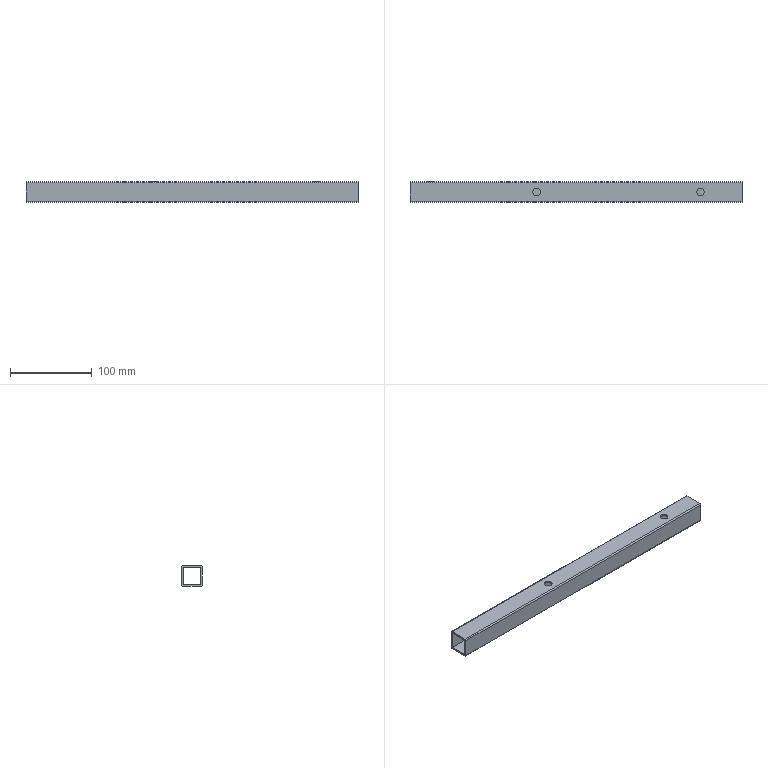Part | NX | features BREP 1 | 1 solid | 20 faces | box 406.4 x 25.4 x 25.4 mm | volume 74121 mm3 | plane 10 | cylinder 10 | commonest cylinder face diameters 9.525 x6 3.175 x4
STEP:
#1=CARTESIAN_POINT('',(-203.2,12.7,-11.113));
#2=VERTEX_POINT('',#1);
#3=CARTESIAN_POINT('',(-203.2,12.7,11.113));
#4=VERTEX_POINT('',#3);
#5=CARTESIAN_POINT('',(-203.2,12.7,-11.113));
#6=DIRECTION('',(0.,0.,1.));
#7=VECTOR('',#6,1000.);
#8=LINE('',#5,#7);
#9=EDGE_CURVE('',#2,#4,#8,.T.);
#10=ORIENTED_EDGE('',*,*,#9,.F.);
#11=CARTESIAN_POINT('',(-203.2,11.113,-12.7));
#12=VERTEX_POINT('',#11);
#13=CARTESIAN_POINT('',(-203.2,11.113,-11.113));
#14=DIRECTION('',(-1.,0.,0.));
#15=DIRECTION('',(0.,1.,0.));
#16=AXIS2_PLACEMENT_3D('',#13,#14,#15);
#17=CIRCLE('',#16,1.587);
#18=EDGE_CURVE('',#2,#12,#17,.T.);
#19=ORIENTED_EDGE('',*,*,#18,.T.);
#20=CARTESIAN_POINT('',(-203.2,-11.113,-12.7));
#21=VERTEX_POINT('',#20);
#22=CARTESIAN_POINT('',(-203.2,-11.113,-12.7));
#23=DIRECTION('',(0.,1.,0.));
#24=VECTOR('',#23,1000.);
#25=LINE('',#22,#24);
#26=EDGE_CURVE('',#21,#12,#25,.T.);
#27=ORIENTED_EDGE('',*,*,#26,.F.);
#28=CARTESIAN_POINT('',(-203.2,-12.7,-11.113));
#29=VERTEX_POINT('',#28);
#30=CARTESIAN_POINT('',(-203.2,-11.113,-11.113));
#31=DIRECTION('',(-1.,0.,0.));
#32=DIRECTION('',(0.,0.,-1.));
#33=AXIS2_PLACEMENT_3D('',#30,#31,#32);
#34=CIRCLE('',#33,1.587);
#35=EDGE_CURVE('',#21,#29,#34,.T.);
#36=ORIENTED_EDGE('',*,*,#35,.T.);
#37=CARTESIAN_POINT('',(-203.2,-12.7,11.113));
#38=VERTEX_POINT('',#37);
#39=CARTESIAN_POINT('',(-203.2,-12.7,11.113));
#40=DIRECTION('',(0.,0.,-1.));
#41=VECTOR('',#40,1000.);
#42=LINE('',#39,#41);
#43=EDGE_CURVE('',#38,#29,#42,.T.);
#44=ORIENTED_EDGE('',*,*,#43,.F.);
#45=CARTESIAN_POINT('',(-203.2,-11.113,12.7));
#46=VERTEX_POINT('',#45);
#47=CARTESIAN_POINT('',(-203.2,-11.113,11.113));
#48=DIRECTION('',(-1.,0.,0.));
#49=DIRECTION('',(0.,-1.,0.));
#50=AXIS2_PLACEMENT_3D('',#47,#48,#49);
#51=CIRCLE('',#50,1.587);
#52=EDGE_CURVE('',#38,#46,#51,.T.);
#53=ORIENTED_EDGE('',*,*,#52,.T.);
#54=CARTESIAN_POINT('',(-203.2,11.113,12.7));
#55=VERTEX_POINT('',#54);
#56=CARTESIAN_POINT('',(-203.2,11.113,12.7));
#57=DIRECTION('',(0.,-1.,0.));
#58=VECTOR('',#57,1000.);
#59=LINE('',#56,#58);
#60=EDGE_CURVE('',#55,#46,#59,.T.);
#61=ORIENTED_EDGE('',*,*,#60,.F.);
#62=CARTESIAN_POINT('',(-203.2,11.113,11.113));
#63=DIRECTION('',(-1.,0.,0.));
#64=DIRECTION('',(0.,0.,1.));
#65=AXIS2_PLACEMENT_3D('',#62,#63,#64);
#66=CIRCLE('',#65,1.587);
#67=EDGE_CURVE('',#55,#4,#66,.T.);
#68=ORIENTED_EDGE('',*,*,#67,.T.);
#69=EDGE_LOOP('',(#10,#19,#27,#36,#44,#53,#61,#68));
#70=FACE_BOUND('',#69,.T.);
#71=CARTESIAN_POINT('',(-203.2,10.719,10.719));
#72=VERTEX_POINT('',#71);
#73=CARTESIAN_POINT('',(-203.2,10.719,-10.719));
#74=VERTEX_POINT('',#73);
#75=CARTESIAN_POINT('',(-203.2,10.719,10.719));
#76=DIRECTION('',(0.,0.,-1.));
#77=VECTOR('',#76,1000.);
#78=LINE('',#75,#77);
#79=EDGE_CURVE('',#72,#74,#78,.T.);
#80=ORIENTED_EDGE('',*,*,#79,.F.);
#81=CARTESIAN_POINT('',(-203.2,-10.719,10.719));
#82=VERTEX_POINT('',#81);
#83=CARTESIAN_POINT('',(-203.2,-10.719,10.719));
#84=DIRECTION('',(0.,1.,0.));
#85=VECTOR('',#84,1000.);
#86=LINE('',#83,#85);
#87=EDGE_CURVE('',#82,#72,#86,.T.);
#88=ORIENTED_EDGE('',*,*,#87,.F.);
#89=CARTESIAN_POINT('',(-203.2,-10.719,-10.719));
#90=VERTEX_POINT('',#89);
#91=CARTESIAN_POINT('',(-203.2,-10.719,-10.719));
#92=DIRECTION('',(0.,0.,1.));
#93=VECTOR('',#92,1000.);
#94=LINE('',#91,#93);
#95=EDGE_CURVE('',#90,#82,#94,.T.);
#96=ORIENTED_EDGE('',*,*,#95,.F.);
#97=CARTESIAN_POINT('',(-203.2,10.719,-10.719));
#98=DIRECTION('',(0.,-1.,0.));
#99=VECTOR('',#98,1000.);
#100=LINE('',#97,#99);
#101=EDGE_CURVE('',#74,#90,#100,.T.);
#102=ORIENTED_EDGE('',*,*,#101,.F.);
#103=EDGE_LOOP('',(#80,#88,#96,#102));
#104=FACE_BOUND('',#103,.T.);
#105=CARTESIAN_POINT('',(-203.2,0.,0.));
#106=DIRECTION('',(1.,0.,0.));
#107=DIRECTION('',(0.,1.,0.));
#108=AXIS2_PLACEMENT_3D('',#105,#106,#107);
#109=PLANE('',#108);
#110=ADVANCED_FACE('',(#70,#104),#109,.F.);
#111=CARTESIAN_POINT('',(203.2,-10.719,-10.719));
#112=VERTEX_POINT('',#111);
#113=CARTESIAN_POINT('',(-203.2,-10.719,-10.719));
#114=DIRECTION('',(1.,0.,0.));
#115=VECTOR('',#114,1000.);
#116=LINE('',#113,#115);
#117=EDGE_CURVE('',#90,#112,#116,.T.);
#118=ORIENTED_EDGE('',*,*,#117,.T.);
#119=CARTESIAN_POINT('',(203.2,10.719,-10.719));
#120=VERTEX_POINT('',#119);
#121=CARTESIAN_POINT('',(203.2,10.719,-10.719));
#122=DIRECTION('',(0.,-1.,0.));
#123=VECTOR('',#122,1000.);
#124=LINE('',#121,#123);
#125=EDGE_CURVE('',#120,#112,#124,.T.);
#126=ORIENTED_EDGE('',*,*,#125,.F.);
#127=CARTESIAN_POINT('',(-203.2,10.719,-10.719));
#128=DIRECTION('',(1.,0.,0.));
#129=VECTOR('',#128,1000.);
#130=LINE('',#127,#129);
#131=EDGE_CURVE('',#74,#120,#130,.T.);
#132=ORIENTED_EDGE('',*,*,#131,.F.);
#133=ORIENTED_EDGE('',*,*,#101,.T.);
#134=EDGE_LOOP('',(#118,#126,#132,#133));
#135=FACE_BOUND('',#134,.T.);
#136=CARTESIAN_POINT('',(-203.2,10.719,-10.719));
#137=DIRECTION('',(0.,0.,1.));
#138=DIRECTION('',(1.,0.,0.));
#139=AXIS2_PLACEMENT_3D('',#136,#137,#138);
#140=PLANE('',#139);
#141=ADVANCED_FACE('',(#135),#140,.T.);
#142=ORIENTED_EDGE('',*,*,#131,.T.);
#143=CARTESIAN_POINT('',(203.2,10.719,10.719));
#144=VERTEX_POINT('',#143);
#145=CARTESIAN_POINT('',(203.2,10.719,10.719));
#146=DIRECTION('',(0.,0.,-1.));
#147=VECTOR('',#146,1000.);
#148=LINE('',#145,#147);
#149=EDGE_CURVE('',#144,#120,#148,.T.);
#150=ORIENTED_EDGE('',*,*,#149,.F.);
#151=CARTESIAN_POINT('',(-203.2,10.719,10.719));
#152=DIRECTION('',(1.,0.,0.));
#153=VECTOR('',#152,1000.);
#154=LINE('',#151,#153);
#155=EDGE_CURVE('',#72,#144,#154,.T.);
#156=ORIENTED_EDGE('',*,*,#155,.F.);
#157=ORIENTED_EDGE('',*,*,#79,.T.);
#158=EDGE_LOOP('',(#142,#150,#156,#157));
#159=FACE_BOUND('',#158,.T.);
#160=CARTESIAN_POINT('',(-182.562,10.719,0.));
#161=VERTEX_POINT('',#160);
#162=CARTESIAN_POINT('',(-173.037,10.719,0.));
#163=VERTEX_POINT('',#162);
#164=CARTESIAN_POINT('',(-177.8,10.719,0.));
#165=DIRECTION('',(0.,-1.,0.));
#166=DIRECTION('',(-1.,0.,0.));
#167=AXIS2_PLACEMENT_3D('',#164,#165,#166);
#168=CIRCLE('',#167,4.763);
#169=EDGE_CURVE('',#161,#163,#168,.T.);
#170=ORIENTED_EDGE('',*,*,#169,.F.);
#171=CARTESIAN_POINT('',(-177.8,10.719,0.));
#172=DIRECTION('',(0.,-1.,0.));
#173=DIRECTION('',(1.,0.,0.));
#174=AXIS2_PLACEMENT_3D('',#171,#172,#173);
#175=CIRCLE('',#174,4.763);
#176=EDGE_CURVE('',#163,#161,#175,.T.);
#177=ORIENTED_EDGE('',*,*,#176,.F.);
#178=EDGE_LOOP('',(#170,#177));
#179=FACE_BOUND('',#178,.T.);
#180=CARTESIAN_POINT('',(-203.2,10.719,10.719));
#181=DIRECTION('',(0.,-1.,0.));
#182=DIRECTION('',(0.,0.,-1.));
#183=AXIS2_PLACEMENT_3D('',#180,#181,#182);
#184=PLANE('',#183);
#185=ADVANCED_FACE('',(#159,#179),#184,.T.);
#186=ORIENTED_EDGE('',*,*,#155,.T.);
#187=CARTESIAN_POINT('',(203.2,-10.719,10.719));
#188=VERTEX_POINT('',#187);
#189=CARTESIAN_POINT('',(203.2,-10.719,10.719));
#190=DIRECTION('',(0.,1.,0.));
#191=VECTOR('',#190,1000.);
#192=LINE('',#189,#191);
#193=EDGE_CURVE('',#188,#144,#192,.T.);
#194=ORIENTED_EDGE('',*,*,#193,.F.);
#195=CARTESIAN_POINT('',(-203.2,-10.719,10.719));
#196=DIRECTION('',(1.,0.,0.));
#197=VECTOR('',#196,1000.);
#198=LINE('',#195,#197);
#199=EDGE_CURVE('',#82,#188,#198,.T.);
#200=ORIENTED_EDGE('',*,*,#199,.F.);
#201=ORIENTED_EDGE('',*,*,#87,.T.);
#202=EDGE_LOOP('',(#186,#194,#200,#201));
#203=FACE_BOUND('',#202,.T.);
#204=CARTESIAN_POINT('',(-43.498,0.,10.719));
#205=VERTEX_POINT('',#204);
#206=CARTESIAN_POINT('',(-53.023,0.,10.719));
#207=VERTEX_POINT('',#206);
#208=CARTESIAN_POINT('',(-48.26,0.,10.719));
#209=DIRECTION('',(0.,0.,-1.));
#210=DIRECTION('',(1.,0.,0.));
#211=AXIS2_PLACEMENT_3D('',#208,#209,#210);
#212=CIRCLE('',#211,4.763);
#213=EDGE_CURVE('',#205,#207,#212,.T.);
#214=ORIENTED_EDGE('',*,*,#213,.F.);
#215=CARTESIAN_POINT('',(-48.26,0.,10.719));
#216=DIRECTION('',(0.,0.,-1.));
#217=DIRECTION('',(-1.,0.,0.));
#218=AXIS2_PLACEMENT_3D('',#215,#216,#217);
#219=CIRCLE('',#218,4.763);
#220=EDGE_CURVE('',#207,#205,#219,.T.);
#221=ORIENTED_EDGE('',*,*,#220,.F.);
#222=EDGE_LOOP('',(#214,#221));
#223=FACE_BOUND('',#222,.T.);
#224=CARTESIAN_POINT('',(157.162,0.,10.719));
#225=VERTEX_POINT('',#224);
#226=CARTESIAN_POINT('',(147.637,0.,10.719));
#227=VERTEX_POINT('',#226);
#228=CARTESIAN_POINT('',(152.4,0.,10.719));
#229=DIRECTION('',(0.,0.,-1.));
#230=DIRECTION('',(1.,0.,0.));
#231=AXIS2_PLACEMENT_3D('',#228,#229,#230);
#232=CIRCLE('',#231,4.763);
#233=EDGE_CURVE('',#225,#227,#232,.T.);
#234=ORIENTED_EDGE('',*,*,#233,.F.);
#235=CARTESIAN_POINT('',(152.4,0.,10.719));
#236=DIRECTION('',(0.,0.,-1.));
#237=DIRECTION('',(-1.,0.,0.));
#238=AXIS2_PLACEMENT_3D('',#235,#236,#237);
#239=CIRCLE('',#238,4.763);
#240=EDGE_CURVE('',#227,#225,#239,.T.);
#241=ORIENTED_EDGE('',*,*,#240,.F.);
#242=EDGE_LOOP('',(#234,#241));
#243=FACE_BOUND('',#242,.T.);
#244=CARTESIAN_POINT('',(-203.2,-10.719,10.719));
#245=DIRECTION('',(0.,0.,-1.));
#246=DIRECTION('',(0.,-1.,0.));
#247=AXIS2_PLACEMENT_3D('',#244,#245,#246);
#248=PLANE('',#247);
#249=ADVANCED_FACE('',(#203,#223,#243),#248,.T.);
#250=ORIENTED_EDGE('',*,*,#199,.T.);
#251=CARTESIAN_POINT('',(203.2,-10.719,-10.719));
#252=DIRECTION('',(0.,0.,1.));
#253=VECTOR('',#252,1000.);
#254=LINE('',#251,#253);
#255=EDGE_CURVE('',#112,#188,#254,.T.);
#256=ORIENTED_EDGE('',*,*,#255,.F.);
#257=ORIENTED_EDGE('',*,*,#117,.F.);
#258=ORIENTED_EDGE('',*,*,#95,.T.);
#259=EDGE_LOOP('',(#250,#256,#257,#258));
#260=FACE_BOUND('',#259,.T.);
#261=CARTESIAN_POINT('',(-203.2,-10.719,-10.719));
#262=DIRECTION('',(0.,1.,0.));
#263=DIRECTION('',(1.,0.,0.));
#264=AXIS2_PLACEMENT_3D('',#261,#262,#263);
#265=PLANE('',#264);
#266=ADVANCED_FACE('',(#260),#265,.T.);
#267=CARTESIAN_POINT('',(203.2,11.113,12.7));
#268=VERTEX_POINT('',#267);
#269=CARTESIAN_POINT('',(203.2,-11.113,12.7));
#270=VERTEX_POINT('',#269);
#271=CARTESIAN_POINT('',(203.2,11.113,12.7));
#272=DIRECTION('',(0.,-1.,0.));
#273=VECTOR('',#272,1000.);
#274=LINE('',#271,#273);
#275=EDGE_CURVE('',#268,#270,#274,.T.);
#276=ORIENTED_EDGE('',*,*,#275,.T.);
#277=CARTESIAN_POINT('',(203.2,-12.7,11.113));
#278=VERTEX_POINT('',#277);
#279=CARTESIAN_POINT('',(203.2,-11.113,11.113));
#280=DIRECTION('',(1.,0.,0.));
#281=DIRECTION('',(0.,0.,1.));
#282=AXIS2_PLACEMENT_3D('',#279,#280,#281);
#283=CIRCLE('',#282,1.587);
#284=EDGE_CURVE('',#270,#278,#283,.T.);
#285=ORIENTED_EDGE('',*,*,#284,.T.);
#286=CARTESIAN_POINT('',(203.2,-12.7,-11.113));
#287=VERTEX_POINT('',#286);
#288=CARTESIAN_POINT('',(203.2,-12.7,11.113));
#289=DIRECTION('',(0.,0.,-1.));
#290=VECTOR('',#289,1000.);
#291=LINE('',#288,#290);
#292=EDGE_CURVE('',#278,#287,#291,.T.);
#293=ORIENTED_EDGE('',*,*,#292,.T.);
#294=CARTESIAN_POINT('',(203.2,-11.113,-12.7));
#295=VERTEX_POINT('',#294);
#296=CARTESIAN_POINT('',(203.2,-11.113,-11.113));
#297=DIRECTION('',(1.,0.,0.));
#298=DIRECTION('',(0.,-1.,0.));
#299=AXIS2_PLACEMENT_3D('',#296,#297,#298);
#300=CIRCLE('',#299,1.587);
#301=EDGE_CURVE('',#287,#295,#300,.T.);
#302=ORIENTED_EDGE('',*,*,#301,.T.);
#303=CARTESIAN_POINT('',(203.2,11.113,-12.7));
#304=VERTEX_POINT('',#303);
#305=CARTESIAN_POINT('',(203.2,-11.113,-12.7));
#306=DIRECTION('',(0.,1.,0.));
#307=VECTOR('',#306,1000.);
#308=LINE('',#305,#307);
#309=EDGE_CURVE('',#295,#304,#308,.T.);
#310=ORIENTED_EDGE('',*,*,#309,.T.);
#311=CARTESIAN_POINT('',(203.2,12.7,-11.113));
#312=VERTEX_POINT('',#311);
#313=CARTESIAN_POINT('',(203.2,11.113,-11.113));
#314=DIRECTION('',(1.,0.,0.));
#315=DIRECTION('',(0.,0.,-1.));
#316=AXIS2_PLACEMENT_3D('',#313,#314,#315);
#317=CIRCLE('',#316,1.587);
#318=EDGE_CURVE('',#304,#312,#317,.T.);
#319=ORIENTED_EDGE('',*,*,#318,.T.);
#320=CARTESIAN_POINT('',(203.2,12.7,11.113));
#321=VERTEX_POINT('',#320);
#322=CARTESIAN_POINT('',(203.2,12.7,-11.113));
#323=DIRECTION('',(0.,0.,1.));
#324=VECTOR('',#323,1000.);
#325=LINE('',#322,#324);
#326=EDGE_CURVE('',#312,#321,#325,.T.);
#327=ORIENTED_EDGE('',*,*,#326,.T.);
#328=CARTESIAN_POINT('',(203.2,11.113,11.113));
#329=DIRECTION('',(1.,0.,0.));
#330=DIRECTION('',(0.,1.,0.));
#331=AXIS2_PLACEMENT_3D('',#328,#329,#330);
#332=CIRCLE('',#331,1.587);
#333=EDGE_CURVE('',#321,#268,#332,.T.);
#334=ORIENTED_EDGE('',*,*,#333,.T.);
#335=EDGE_LOOP('',(#276,#285,#293,#302,#310,#319,#327,#334));
#336=FACE_BOUND('',#335,.T.);
#337=ORIENTED_EDGE('',*,*,#255,.T.);
#338=ORIENTED_EDGE('',*,*,#193,.T.);
#339=ORIENTED_EDGE('',*,*,#149,.T.);
#340=ORIENTED_EDGE('',*,*,#125,.T.);
#341=EDGE_LOOP('',(#337,#338,#339,#340));
#342=FACE_BOUND('',#341,.T.);
#343=CARTESIAN_POINT('',(203.2,0.,0.));
#344=DIRECTION('',(1.,0.,0.));
#345=DIRECTION('',(0.,1.,0.));
#346=AXIS2_PLACEMENT_3D('',#343,#344,#345);
#347=PLANE('',#346);
#348=ADVANCED_FACE('',(#336,#342),#347,.T.);
#349=ORIENTED_EDGE('',*,*,#333,.F.);
#350=CARTESIAN_POINT('',(203.2,12.7,11.113));
#351=DIRECTION('',(-1.,0.,0.));
#352=VECTOR('',#351,1000.);
#353=LINE('',#350,#352);
#354=EDGE_CURVE('',#321,#4,#353,.T.);
#355=ORIENTED_EDGE('',*,*,#354,.T.);
#356=ORIENTED_EDGE('',*,*,#67,.F.);
#357=CARTESIAN_POINT('',(203.2,11.113,12.7));
#358=DIRECTION('',(-1.,0.,0.));
#359=VECTOR('',#358,1000.);
#360=LINE('',#357,#359);
#361=EDGE_CURVE('',#268,#55,#360,.T.);
#362=ORIENTED_EDGE('',*,*,#361,.F.);
#363=EDGE_LOOP('',(#349,#355,#356,#362));
#364=FACE_BOUND('',#363,.T.);
#365=CARTESIAN_POINT('',(203.838,11.113,11.113));
#366=DIRECTION('',(-1.,0.,0.));
#367=DIRECTION('',(0.,0.,1.));
#368=AXIS2_PLACEMENT_3D('',#365,#366,#367);
#369=CYLINDRICAL_SURFACE('',#368,1.587);
#370=ADVANCED_FACE('',(#364),#369,.T.);
#371=ORIENTED_EDGE('',*,*,#60,.T.);
#372=CARTESIAN_POINT('',(203.2,-11.113,12.7));
#373=DIRECTION('',(-1.,0.,0.));
#374=VECTOR('',#373,1000.);
#375=LINE('',#372,#374);
#376=EDGE_CURVE('',#270,#46,#375,.T.);
#377=ORIENTED_EDGE('',*,*,#376,.F.);
#378=ORIENTED_EDGE('',*,*,#275,.F.);
#379=ORIENTED_EDGE('',*,*,#361,.T.);
#380=EDGE_LOOP('',(#371,#377,#378,#379));
#381=FACE_BOUND('',#380,.T.);
#382=CARTESIAN_POINT('',(-43.498,0.,12.7));
#383=VERTEX_POINT('',#382);
#384=CARTESIAN_POINT('',(-53.023,0.,12.7));
#385=VERTEX_POINT('',#384);
#386=CARTESIAN_POINT('',(-48.26,0.,12.7));
#387=DIRECTION('',(0.,0.,-1.));
#388=DIRECTION('',(1.,0.,0.));
#389=AXIS2_PLACEMENT_3D('',#386,#387,#388);
#390=CIRCLE('',#389,4.763);
#391=EDGE_CURVE('',#383,#385,#390,.T.);
#392=ORIENTED_EDGE('',*,*,#391,.T.);
#393=CARTESIAN_POINT('',(-48.26,0.,12.7));
#394=DIRECTION('',(0.,0.,-1.));
#395=DIRECTION('',(-1.,0.,0.));
#396=AXIS2_PLACEMENT_3D('',#393,#394,#395);
#397=CIRCLE('',#396,4.763);
#398=EDGE_CURVE('',#385,#383,#397,.T.);
#399=ORIENTED_EDGE('',*,*,#398,.T.);
#400=EDGE_LOOP('',(#392,#399));
#401=FACE_BOUND('',#400,.T.);
#402=CARTESIAN_POINT('',(157.162,0.,12.7));
#403=VERTEX_POINT('',#402);
#404=CARTESIAN_POINT('',(147.637,0.,12.7));
#405=VERTEX_POINT('',#404);
#406=CARTESIAN_POINT('',(152.4,0.,12.7));
#407=DIRECTION('',(0.,0.,-1.));
#408=DIRECTION('',(1.,0.,0.));
#409=AXIS2_PLACEMENT_3D('',#406,#407,#408);
#410=CIRCLE('',#409,4.763);
#411=EDGE_CURVE('',#403,#405,#410,.T.);
#412=ORIENTED_EDGE('',*,*,#411,.T.);
#413=CARTESIAN_POINT('',(152.4,0.,12.7));
#414=DIRECTION('',(0.,0.,-1.));
#415=DIRECTION('',(-1.,0.,0.));
#416=AXIS2_PLACEMENT_3D('',#413,#414,#415);
#417=CIRCLE('',#416,4.763);
#418=EDGE_CURVE('',#405,#403,#417,.T.);
#419=ORIENTED_EDGE('',*,*,#418,.T.);
#420=EDGE_LOOP('',(#412,#419));
#421=FACE_BOUND('',#420,.T.);
#422=CARTESIAN_POINT('',(-203.2,12.7,12.7));
#423=DIRECTION('',(0.,0.,1.));
#424=DIRECTION('',(1.,0.,0.));
#425=AXIS2_PLACEMENT_3D('',#422,#423,#424);
#426=PLANE('',#425);
#427=ADVANCED_FACE('',(#381,#401,#421),#426,.T.);
#428=ORIENTED_EDGE('',*,*,#284,.F.);
#429=ORIENTED_EDGE('',*,*,#376,.T.);
#430=ORIENTED_EDGE('',*,*,#52,.F.);
#431=CARTESIAN_POINT('',(203.2,-12.7,11.113));
#432=DIRECTION('',(-1.,0.,0.));
#433=VECTOR('',#432,1000.);
#434=LINE('',#431,#433);
#435=EDGE_CURVE('',#278,#38,#434,.T.);
#436=ORIENTED_EDGE('',*,*,#435,.F.);
#437=EDGE_LOOP('',(#428,#429,#430,#436));
#438=FACE_BOUND('',#437,.T.);
#439=CARTESIAN_POINT('',(203.838,-11.113,11.113));
#440=DIRECTION('',(-1.,0.,0.));
#441=DIRECTION('',(0.,-1.,0.));
#442=AXIS2_PLACEMENT_3D('',#439,#440,#441);
#443=CYLINDRICAL_SURFACE('',#442,1.587);
#444=ADVANCED_FACE('',(#438),#443,.T.);
#445=ORIENTED_EDGE('',*,*,#43,.T.);
#446=CARTESIAN_POINT('',(203.2,-12.7,-11.113));
#447=DIRECTION('',(-1.,0.,0.));
#448=VECTOR('',#447,1000.);
#449=LINE('',#446,#448);
#450=EDGE_CURVE('',#287,#29,#449,.T.);
#451=ORIENTED_EDGE('',*,*,#450,.F.);
#452=ORIENTED_EDGE('',*,*,#292,.F.);
#453=ORIENTED_EDGE('',*,*,#435,.T.);
#454=EDGE_LOOP('',(#445,#451,#452,#453));
#455=FACE_BOUND('',#454,.T.);
#456=CARTESIAN_POINT('',(-203.2,-12.7,12.7));
#457=DIRECTION('',(0.,-1.,0.));
#458=DIRECTION('',(0.,0.,-1.));
#459=AXIS2_PLACEMENT_3D('',#456,#457,#458);
#460=PLANE('',#459);
#461=ADVANCED_FACE('',(#455),#460,.T.);
#462=ORIENTED_EDGE('',*,*,#301,.F.);
#463=ORIENTED_EDGE('',*,*,#450,.T.);
#464=ORIENTED_EDGE('',*,*,#35,.F.);
#465=CARTESIAN_POINT('',(203.2,-11.113,-12.7));
#466=DIRECTION('',(-1.,0.,0.));
#467=VECTOR('',#466,1000.);
#468=LINE('',#465,#467);
#469=EDGE_CURVE('',#295,#21,#468,.T.);
#470=ORIENTED_EDGE('',*,*,#469,.F.);
#471=EDGE_LOOP('',(#462,#463,#464,#470));
#472=FACE_BOUND('',#471,.T.);
#473=CARTESIAN_POINT('',(203.838,-11.113,-11.113));
#474=DIRECTION('',(-1.,0.,0.));
#475=DIRECTION('',(0.,0.,-1.));
#476=AXIS2_PLACEMENT_3D('',#473,#474,#475);
#477=CYLINDRICAL_SURFACE('',#476,1.587);
#478=ADVANCED_FACE('',(#472),#477,.T.);
#479=ORIENTED_EDGE('',*,*,#309,.F.);
#480=ORIENTED_EDGE('',*,*,#469,.T.);
#481=ORIENTED_EDGE('',*,*,#26,.T.);
#482=CARTESIAN_POINT('',(203.2,11.113,-12.7));
#483=DIRECTION('',(-1.,0.,0.));
#484=VECTOR('',#483,1000.);
#485=LINE('',#482,#484);
#486=EDGE_CURVE('',#304,#12,#485,.T.);
#487=ORIENTED_EDGE('',*,*,#486,.F.);
#488=EDGE_LOOP('',(#479,#480,#481,#487));
#489=FACE_BOUND('',#488,.T.);
#490=CARTESIAN_POINT('',(-203.2,-12.7,-12.7));
#491=DIRECTION('',(0.,0.,-1.));
#492=DIRECTION('',(0.,-1.,0.));
#493=AXIS2_PLACEMENT_3D('',#490,#491,#492);
#494=PLANE('',#493);
#495=ADVANCED_FACE('',(#489),#494,.T.);
#496=ORIENTED_EDGE('',*,*,#318,.F.);
#497=ORIENTED_EDGE('',*,*,#486,.T.);
#498=ORIENTED_EDGE('',*,*,#18,.F.);
#499=CARTESIAN_POINT('',(203.2,12.7,-11.113));
#500=DIRECTION('',(-1.,0.,0.));
#501=VECTOR('',#500,1000.);
#502=LINE('',#499,#501);
#503=EDGE_CURVE('',#312,#2,#502,.T.);
#504=ORIENTED_EDGE('',*,*,#503,.F.);
#505=EDGE_LOOP('',(#496,#497,#498,#504));
#506=FACE_BOUND('',#505,.T.);
#507=CARTESIAN_POINT('',(203.838,11.113,-11.113));
#508=DIRECTION('',(-1.,0.,0.));
#509=DIRECTION('',(0.,1.,0.));
#510=AXIS2_PLACEMENT_3D('',#507,#508,#509);
#511=CYLINDRICAL_SURFACE('',#510,1.587);
#512=ADVANCED_FACE('',(#506),#511,.T.);
#513=ORIENTED_EDGE('',*,*,#326,.F.);
#514=ORIENTED_EDGE('',*,*,#503,.T.);
#515=ORIENTED_EDGE('',*,*,#9,.T.);
#516=ORIENTED_EDGE('',*,*,#354,.F.);
#517=EDGE_LOOP('',(#513,#514,#515,#516));
#518=FACE_BOUND('',#517,.T.);
#519=CARTESIAN_POINT('',(-182.562,12.7,0.));
#520=VERTEX_POINT('',#519);
#521=CARTESIAN_POINT('',(-173.037,12.7,0.));
#522=VERTEX_POINT('',#521);
#523=CARTESIAN_POINT('',(-177.8,12.7,0.));
#524=DIRECTION('',(0.,-1.,0.));
#525=DIRECTION('',(-1.,0.,0.));
#526=AXIS2_PLACEMENT_3D('',#523,#524,#525);
#527=CIRCLE('',#526,4.763);
#528=EDGE_CURVE('',#520,#522,#527,.T.);
#529=ORIENTED_EDGE('',*,*,#528,.T.);
#530=CARTESIAN_POINT('',(-177.8,12.7,0.));
#531=DIRECTION('',(0.,-1.,0.));
#532=DIRECTION('',(1.,0.,0.));
#533=AXIS2_PLACEMENT_3D('',#530,#531,#532);
#534=CIRCLE('',#533,4.763);
#535=EDGE_CURVE('',#522,#520,#534,.T.);
#536=ORIENTED_EDGE('',*,*,#535,.T.);
#537=EDGE_LOOP('',(#529,#536));
#538=FACE_BOUND('',#537,.T.);
#539=CARTESIAN_POINT('',(-203.2,12.7,-12.7));
#540=DIRECTION('',(0.,1.,0.));
#541=DIRECTION('',(1.,0.,0.));
#542=AXIS2_PLACEMENT_3D('',#539,#540,#541);
#543=PLANE('',#542);
#544=ADVANCED_FACE('',(#518,#538),#543,.T.);
#545=CARTESIAN_POINT('',(-173.037,12.7,0.));
#546=DIRECTION('',(0.,-1.,0.));
#547=VECTOR('',#546,1000.);
#548=LINE('',#545,#547);
#549=EDGE_CURVE('',#163,#522,#548,.F.);
#550=ORIENTED_EDGE('',*,*,#549,.F.);
#551=ORIENTED_EDGE('',*,*,#176,.T.);
#552=CARTESIAN_POINT('',(-182.562,12.7,0.));
#553=DIRECTION('',(0.,-1.,0.));
#554=VECTOR('',#553,1000.);
#555=LINE('',#552,#554);
#556=EDGE_CURVE('',#161,#520,#555,.F.);
#557=ORIENTED_EDGE('',*,*,#556,.T.);
#558=ORIENTED_EDGE('',*,*,#535,.F.);
#559=EDGE_LOOP('',(#550,#551,#557,#558));
#560=FACE_BOUND('',#559,.T.);
#561=CARTESIAN_POINT('',(-177.8,12.7,0.));
#562=DIRECTION('',(0.,-1.,0.));
#563=DIRECTION('',(1.,0.,0.));
#564=AXIS2_PLACEMENT_3D('',#561,#562,#563);
#565=CYLINDRICAL_SURFACE('',#564,4.763);
#566=ADVANCED_FACE('',(#560),#565,.F.);
#567=ORIENTED_EDGE('',*,*,#556,.F.);
#568=ORIENTED_EDGE('',*,*,#169,.T.);
#569=ORIENTED_EDGE('',*,*,#549,.T.);
#570=ORIENTED_EDGE('',*,*,#528,.F.);
#571=EDGE_LOOP('',(#567,#568,#569,#570));
#572=FACE_BOUND('',#571,.T.);
#573=CARTESIAN_POINT('',(-177.8,12.7,0.));
#574=DIRECTION('',(0.,-1.,0.));
#575=DIRECTION('',(1.,0.,0.));
#576=AXIS2_PLACEMENT_3D('',#573,#574,#575);
#577=CYLINDRICAL_SURFACE('',#576,4.763);
#578=ADVANCED_FACE('',(#572),#577,.F.);
#579=CARTESIAN_POINT('',(-53.023,0.,12.7));
#580=DIRECTION('',(0.,0.,-1.));
#581=VECTOR('',#580,1000.);
#582=LINE('',#579,#581);
#583=EDGE_CURVE('',#385,#207,#582,.T.);
#584=ORIENTED_EDGE('',*,*,#583,.T.);
#585=ORIENTED_EDGE('',*,*,#220,.T.);
#586=CARTESIAN_POINT('',(-43.498,0.,12.7));
#587=DIRECTION('',(0.,0.,-1.));
#588=VECTOR('',#587,1000.);
#589=LINE('',#586,#588);
#590=EDGE_CURVE('',#383,#205,#589,.T.);
#591=ORIENTED_EDGE('',*,*,#590,.F.);
#592=ORIENTED_EDGE('',*,*,#398,.F.);
#593=EDGE_LOOP('',(#584,#585,#591,#592));
#594=FACE_BOUND('',#593,.T.);
#595=CARTESIAN_POINT('',(-48.26,0.,12.7));
#596=DIRECTION('',(0.,0.,-1.));
#597=DIRECTION('',(-1.,0.,0.));
#598=AXIS2_PLACEMENT_3D('',#595,#596,#597);
#599=CYLINDRICAL_SURFACE('',#598,4.763);
#600=ADVANCED_FACE('',(#594),#599,.F.);
#601=ORIENTED_EDGE('',*,*,#590,.T.);
#602=ORIENTED_EDGE('',*,*,#213,.T.);
#603=ORIENTED_EDGE('',*,*,#583,.F.);
#604=ORIENTED_EDGE('',*,*,#391,.F.);
#605=EDGE_LOOP('',(#601,#602,#603,#604));
#606=FACE_BOUND('',#605,.T.);
#607=CARTESIAN_POINT('',(-48.26,0.,12.7));
#608=DIRECTION('',(0.,0.,-1.));
#609=DIRECTION('',(-1.,0.,0.));
#610=AXIS2_PLACEMENT_3D('',#607,#608,#609);
#611=CYLINDRICAL_SURFACE('',#610,4.763);
#612=ADVANCED_FACE('',(#606),#611,.F.);
#613=CARTESIAN_POINT('',(147.637,0.,12.7));
#614=DIRECTION('',(0.,0.,-1.));
#615=VECTOR('',#614,1000.);
#616=LINE('',#613,#615);
#617=EDGE_CURVE('',#405,#227,#616,.T.);
#618=ORIENTED_EDGE('',*,*,#617,.T.);
#619=ORIENTED_EDGE('',*,*,#240,.T.);
#620=CARTESIAN_POINT('',(157.162,0.,12.7));
#621=DIRECTION('',(0.,0.,-1.));
#622=VECTOR('',#621,1000.);
#623=LINE('',#620,#622);
#624=EDGE_CURVE('',#403,#225,#623,.T.);
#625=ORIENTED_EDGE('',*,*,#624,.F.);
#626=ORIENTED_EDGE('',*,*,#418,.F.);
#627=EDGE_LOOP('',(#618,#619,#625,#626));
#628=FACE_BOUND('',#627,.T.);
#629=CARTESIAN_POINT('',(152.4,0.,12.7));
#630=DIRECTION('',(0.,0.,-1.));
#631=DIRECTION('',(-1.,0.,0.));
#632=AXIS2_PLACEMENT_3D('',#629,#630,#631);
#633=CYLINDRICAL_SURFACE('',#632,4.763);
#634=ADVANCED_FACE('',(#628),#633,.F.);
#635=ORIENTED_EDGE('',*,*,#624,.T.);
#636=ORIENTED_EDGE('',*,*,#233,.T.);
#637=ORIENTED_EDGE('',*,*,#617,.F.);
#638=ORIENTED_EDGE('',*,*,#411,.F.);
#639=EDGE_LOOP('',(#635,#636,#637,#638));
#640=FACE_BOUND('',#639,.T.);
#641=CARTESIAN_POINT('',(152.4,0.,12.7));
#642=DIRECTION('',(0.,0.,-1.));
#643=DIRECTION('',(-1.,0.,0.));
#644=AXIS2_PLACEMENT_3D('',#641,#642,#643);
#645=CYLINDRICAL_SURFACE('',#644,4.763);
#646=ADVANCED_FACE('',(#640),#645,.F.);
#647=CLOSED_SHELL('',(#110,#141,#185,#249,#266,#348,#370,#427,#444,#461,#478,#495,#512,#544,#566,#578,#600,#612,#634,#646));
#648=MANIFOLD_SOLID_BREP('',#647);
#649=(LENGTH_UNIT()NAMED_UNIT(*)SI_UNIT(.MILLI.,.METRE.));
#650=UNCERTAINTY_MEASURE_WITH_UNIT(LENGTH_MEASURE(0.00001),#649,'','');
#651=(NAMED_UNIT(*)PLANE_ANGLE_UNIT()SI_UNIT($,.RADIAN.));
#652=(NAMED_UNIT(*)SI_UNIT($,.STERADIAN.)SOLID_ANGLE_UNIT());
#653=(GEOMETRIC_REPRESENTATION_CONTEXT(3)GLOBAL_UNCERTAINTY_ASSIGNED_CONTEXT((#650))GLOBAL_UNIT_ASSIGNED_CONTEXT((#649,#651,#652))REPRESENTATION_CONTEXT('',''));
#654=ADVANCED_BREP_SHAPE_REPRESENTATION('',(#648),#653);